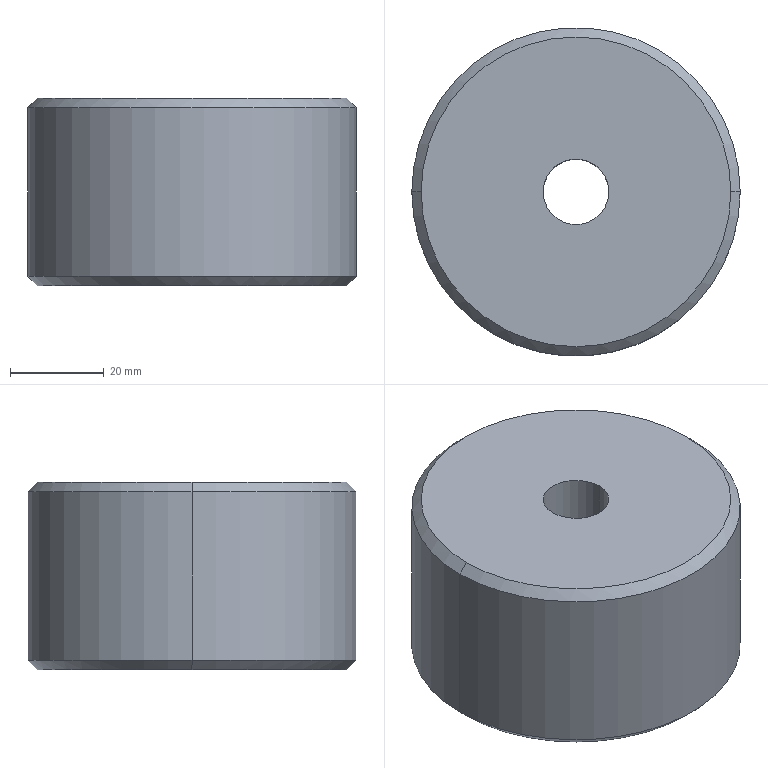Part | SolidWorks | features Chamfer 1, Extrusion 1, HoleWzd 1 | 1 solid | 10 faces | box 70 x 70 x 40 mm | volume 146918 mm3 | cylinder 4 | cone 4 | plane 2 | commonest cylinder face diameters 14 x2 70 x2
STEP:
#1=CARTESIAN_POINT('',(-7.,0.,0.));
#2=VERTEX_POINT('',#1);
#3=CARTESIAN_POINT('',(7.,0.,0.));
#4=VERTEX_POINT('',#3);
#5=CARTESIAN_POINT('',(0.,0.,0.));
#6=DIRECTION('',(0.,0.,1.));
#7=DIRECTION('',(1.,0.,0.));
#8=AXIS2_PLACEMENT_3D('',#5,#6,#7);
#9=CIRCLE('',#8,7.);
#10=EDGE_CURVE('',#2,#4,#9,.T.);
#11=ORIENTED_EDGE('',*,*,#10,.F.);
#12=CARTESIAN_POINT('',(-7.,0.,40.));
#13=VERTEX_POINT('',#12);
#14=CARTESIAN_POINT('',(-7.,0.,40.));
#15=DIRECTION('',(0.,0.,1.));
#16=VECTOR('',#15,1000.);
#17=LINE('',#14,#16);
#18=EDGE_CURVE('',#2,#13,#17,.T.);
#19=ORIENTED_EDGE('',*,*,#18,.T.);
#20=CARTESIAN_POINT('',(7.,0.,40.));
#21=VERTEX_POINT('',#20);
#22=CARTESIAN_POINT('',(0.,0.,40.));
#23=DIRECTION('',(0.,0.,1.));
#24=DIRECTION('',(1.,0.,0.));
#25=AXIS2_PLACEMENT_3D('',#22,#23,#24);
#26=CIRCLE('',#25,7.);
#27=EDGE_CURVE('',#13,#21,#26,.T.);
#28=ORIENTED_EDGE('',*,*,#27,.T.);
#29=CARTESIAN_POINT('',(7.,0.,40.));
#30=DIRECTION('',(0.,0.,1.));
#31=VECTOR('',#30,1000.);
#32=LINE('',#29,#31);
#33=EDGE_CURVE('',#4,#21,#32,.T.);
#34=ORIENTED_EDGE('',*,*,#33,.F.);
#35=EDGE_LOOP('',(#11,#19,#28,#34));
#36=FACE_OUTER_BOUND('',#35,.T.);
#37=CARTESIAN_POINT('',(0.,0.,40.));
#38=DIRECTION('',(0.,0.,1.));
#39=DIRECTION('',(1.,0.,0.));
#40=AXIS2_PLACEMENT_3D('',#37,#38,#39);
#41=CYLINDRICAL_SURFACE('',#40,7.);
#42=ADVANCED_FACE('',(#36),#41,.F.);
#43=CARTESIAN_POINT('',(33.,0.,40.));
#44=VERTEX_POINT('',#43);
#45=CARTESIAN_POINT('',(-33.,0.,40.));
#46=VERTEX_POINT('',#45);
#47=CARTESIAN_POINT('',(0.,0.,40.));
#48=DIRECTION('',(0.,0.,1.));
#49=DIRECTION('',(1.,0.,0.));
#50=AXIS2_PLACEMENT_3D('',#47,#48,#49);
#51=CIRCLE('',#50,33.);
#52=EDGE_CURVE('',#44,#46,#51,.T.);
#53=ORIENTED_EDGE('',*,*,#52,.F.);
#54=CARTESIAN_POINT('',(35.,0.,38.));
#55=VERTEX_POINT('',#54);
#56=CARTESIAN_POINT('',(33.,0.,40.));
#57=DIRECTION('',(0.7071,0.,-0.7071));
#58=VECTOR('',#57,1000.);
#59=LINE('',#56,#58);
#60=EDGE_CURVE('',#44,#55,#59,.T.);
#61=ORIENTED_EDGE('',*,*,#60,.T.);
#62=CARTESIAN_POINT('',(-35.,0.,38.));
#63=VERTEX_POINT('',#62);
#64=CARTESIAN_POINT('',(0.,0.,38.));
#65=DIRECTION('',(0.,0.,-1.));
#66=DIRECTION('',(1.,0.,0.));
#67=AXIS2_PLACEMENT_3D('',#64,#65,#66);
#68=CIRCLE('',#67,35.);
#69=EDGE_CURVE('',#63,#55,#68,.T.);
#70=ORIENTED_EDGE('',*,*,#69,.F.);
#71=CARTESIAN_POINT('',(-33.,0.,40.));
#72=DIRECTION('',(-0.7071,0.,-0.7071));
#73=VECTOR('',#72,1000.);
#74=LINE('',#71,#73);
#75=EDGE_CURVE('',#46,#63,#74,.T.);
#76=ORIENTED_EDGE('',*,*,#75,.F.);
#77=EDGE_LOOP('',(#53,#61,#70,#76));
#78=FACE_OUTER_BOUND('',#77,.T.);
#79=CARTESIAN_POINT('',(0.,0.,40.));
#80=DIRECTION('',(0.,0.,-1.));
#81=DIRECTION('',(-1.,0.,0.));
#82=AXIS2_PLACEMENT_3D('',#79,#80,#81);
#83=CONICAL_SURFACE('',#82,33.,0.7854);
#84=ADVANCED_FACE('',(#78),#83,.T.);
#85=CARTESIAN_POINT('',(-33.,0.,0.));
#86=VERTEX_POINT('',#85);
#87=CARTESIAN_POINT('',(33.,0.,0.));
#88=VERTEX_POINT('',#87);
#89=CARTESIAN_POINT('',(0.,0.,0.));
#90=DIRECTION('',(0.,0.,-1.));
#91=DIRECTION('',(1.,0.,0.));
#92=AXIS2_PLACEMENT_3D('',#89,#90,#91);
#93=CIRCLE('',#92,33.);
#94=EDGE_CURVE('',#86,#88,#93,.T.);
#95=ORIENTED_EDGE('',*,*,#94,.F.);
#96=CARTESIAN_POINT('',(-35.,0.,2.));
#97=VERTEX_POINT('',#96);
#98=CARTESIAN_POINT('',(-35.,0.,2.));
#99=DIRECTION('',(-0.7071,0.,0.7071));
#100=VECTOR('',#99,1000.);
#101=LINE('',#98,#100);
#102=EDGE_CURVE('',#86,#97,#101,.T.);
#103=ORIENTED_EDGE('',*,*,#102,.T.);
#104=CARTESIAN_POINT('',(35.,0.,2.));
#105=VERTEX_POINT('',#104);
#106=CARTESIAN_POINT('',(0.,0.,2.));
#107=DIRECTION('',(0.,0.,1.));
#108=DIRECTION('',(1.,0.,0.));
#109=AXIS2_PLACEMENT_3D('',#106,#107,#108);
#110=CIRCLE('',#109,35.);
#111=EDGE_CURVE('',#105,#97,#110,.T.);
#112=ORIENTED_EDGE('',*,*,#111,.F.);
#113=CARTESIAN_POINT('',(35.,0.,2.));
#114=DIRECTION('',(0.7071,0.,0.7071));
#115=VECTOR('',#114,1000.);
#116=LINE('',#113,#115);
#117=EDGE_CURVE('',#88,#105,#116,.T.);
#118=ORIENTED_EDGE('',*,*,#117,.F.);
#119=EDGE_LOOP('',(#95,#103,#112,#118));
#120=FACE_OUTER_BOUND('',#119,.T.);
#121=CARTESIAN_POINT('',(0.,0.,2.));
#122=DIRECTION('',(0.,0.,1.));
#123=DIRECTION('',(1.,0.,0.));
#124=AXIS2_PLACEMENT_3D('',#121,#122,#123);
#125=CONICAL_SURFACE('',#124,35.,0.7854);
#126=ADVANCED_FACE('',(#120),#125,.T.);
#127=ORIENTED_EDGE('',*,*,#69,.T.);
#128=CARTESIAN_POINT('',(35.,0.,40.));
#129=DIRECTION('',(0.,0.,-1.));
#130=VECTOR('',#129,1000.);
#131=LINE('',#128,#130);
#132=EDGE_CURVE('',#55,#105,#131,.T.);
#133=ORIENTED_EDGE('',*,*,#132,.T.);
#134=ORIENTED_EDGE('',*,*,#111,.T.);
#135=CARTESIAN_POINT('',(-35.,0.,40.));
#136=DIRECTION('',(0.,0.,-1.));
#137=VECTOR('',#136,1000.);
#138=LINE('',#135,#137);
#139=EDGE_CURVE('',#63,#97,#138,.T.);
#140=ORIENTED_EDGE('',*,*,#139,.F.);
#141=EDGE_LOOP('',(#127,#133,#134,#140));
#142=FACE_OUTER_BOUND('',#141,.T.);
#143=CARTESIAN_POINT('',(0.,0.,40.));
#144=DIRECTION('',(0.,0.,-1.));
#145=DIRECTION('',(-1.,0.,0.));
#146=AXIS2_PLACEMENT_3D('',#143,#144,#145);
#147=CYLINDRICAL_SURFACE('',#146,35.);
#148=ADVANCED_FACE('',(#142),#147,.T.);
#149=ORIENTED_EDGE('',*,*,#132,.F.);
#150=CARTESIAN_POINT('',(0.,0.,38.));
#151=DIRECTION('',(0.,0.,-1.));
#152=DIRECTION('',(1.,0.,0.));
#153=AXIS2_PLACEMENT_3D('',#150,#151,#152);
#154=CIRCLE('',#153,35.);
#155=EDGE_CURVE('',#55,#63,#154,.T.);
#156=ORIENTED_EDGE('',*,*,#155,.T.);
#157=ORIENTED_EDGE('',*,*,#139,.T.);
#158=CARTESIAN_POINT('',(0.,0.,2.));
#159=DIRECTION('',(0.,0.,1.));
#160=DIRECTION('',(1.,0.,0.));
#161=AXIS2_PLACEMENT_3D('',#158,#159,#160);
#162=CIRCLE('',#161,35.);
#163=EDGE_CURVE('',#97,#105,#162,.T.);
#164=ORIENTED_EDGE('',*,*,#163,.T.);
#165=EDGE_LOOP('',(#149,#156,#157,#164));
#166=FACE_OUTER_BOUND('',#165,.T.);
#167=CARTESIAN_POINT('',(0.,0.,40.));
#168=DIRECTION('',(0.,0.,-1.));
#169=DIRECTION('',(-1.,0.,0.));
#170=AXIS2_PLACEMENT_3D('',#167,#168,#169);
#171=CYLINDRICAL_SURFACE('',#170,35.);
#172=ADVANCED_FACE('',(#166),#171,.T.);
#173=CARTESIAN_POINT('',(0.,0.,40.));
#174=DIRECTION('',(0.,0.,1.));
#175=DIRECTION('',(1.,0.,0.));
#176=AXIS2_PLACEMENT_3D('',#173,#174,#175);
#177=CIRCLE('',#176,7.);
#178=EDGE_CURVE('',#21,#13,#177,.T.);
#179=ORIENTED_EDGE('',*,*,#178,.F.);
#180=ORIENTED_EDGE('',*,*,#27,.F.);
#181=EDGE_LOOP('',(#179,#180));
#182=FACE_BOUND('',#181,.T.);
#183=CARTESIAN_POINT('',(0.,0.,40.));
#184=DIRECTION('',(0.,0.,1.));
#185=DIRECTION('',(1.,0.,0.));
#186=AXIS2_PLACEMENT_3D('',#183,#184,#185);
#187=CIRCLE('',#186,33.);
#188=EDGE_CURVE('',#46,#44,#187,.T.);
#189=ORIENTED_EDGE('',*,*,#188,.T.);
#190=ORIENTED_EDGE('',*,*,#52,.T.);
#191=EDGE_LOOP('',(#189,#190));
#192=FACE_OUTER_BOUND('',#191,.T.);
#193=CARTESIAN_POINT('',(0.,0.,40.));
#194=DIRECTION('',(0.,0.,1.));
#195=DIRECTION('',(1.,0.,0.));
#196=AXIS2_PLACEMENT_3D('',#193,#194,#195);
#197=PLANE('',#196);
#198=ADVANCED_FACE('',(#182,#192),#197,.T.);
#199=CARTESIAN_POINT('',(0.,0.,0.));
#200=DIRECTION('',(0.,0.,1.));
#201=DIRECTION('',(1.,0.,0.));
#202=AXIS2_PLACEMENT_3D('',#199,#200,#201);
#203=CIRCLE('',#202,7.);
#204=EDGE_CURVE('',#4,#2,#203,.T.);
#205=ORIENTED_EDGE('',*,*,#204,.T.);
#206=ORIENTED_EDGE('',*,*,#10,.T.);
#207=EDGE_LOOP('',(#205,#206));
#208=FACE_BOUND('',#207,.T.);
#209=CARTESIAN_POINT('',(0.,0.,0.));
#210=DIRECTION('',(0.,0.,-1.));
#211=DIRECTION('',(1.,0.,0.));
#212=AXIS2_PLACEMENT_3D('',#209,#210,#211);
#213=CIRCLE('',#212,33.);
#214=EDGE_CURVE('',#88,#86,#213,.T.);
#215=ORIENTED_EDGE('',*,*,#214,.T.);
#216=ORIENTED_EDGE('',*,*,#94,.T.);
#217=EDGE_LOOP('',(#215,#216));
#218=FACE_OUTER_BOUND('',#217,.T.);
#219=CARTESIAN_POINT('',(0.,0.,0.));
#220=DIRECTION('',(0.,0.,1.));
#221=DIRECTION('',(1.,0.,0.));
#222=AXIS2_PLACEMENT_3D('',#219,#220,#221);
#223=PLANE('',#222);
#224=ADVANCED_FACE('',(#208,#218),#223,.F.);
#225=ORIENTED_EDGE('',*,*,#102,.F.);
#226=ORIENTED_EDGE('',*,*,#214,.F.);
#227=ORIENTED_EDGE('',*,*,#117,.T.);
#228=ORIENTED_EDGE('',*,*,#163,.F.);
#229=EDGE_LOOP('',(#225,#226,#227,#228));
#230=FACE_OUTER_BOUND('',#229,.T.);
#231=CARTESIAN_POINT('',(0.,0.,2.));
#232=DIRECTION('',(0.,0.,1.));
#233=DIRECTION('',(1.,0.,0.));
#234=AXIS2_PLACEMENT_3D('',#231,#232,#233);
#235=CONICAL_SURFACE('',#234,35.,0.7854);
#236=ADVANCED_FACE('',(#230),#235,.T.);
#237=ORIENTED_EDGE('',*,*,#60,.F.);
#238=ORIENTED_EDGE('',*,*,#188,.F.);
#239=ORIENTED_EDGE('',*,*,#75,.T.);
#240=ORIENTED_EDGE('',*,*,#155,.F.);
#241=EDGE_LOOP('',(#237,#238,#239,#240));
#242=FACE_OUTER_BOUND('',#241,.T.);
#243=CARTESIAN_POINT('',(0.,0.,40.));
#244=DIRECTION('',(0.,0.,-1.));
#245=DIRECTION('',(-1.,0.,0.));
#246=AXIS2_PLACEMENT_3D('',#243,#244,#245);
#247=CONICAL_SURFACE('',#246,33.,0.7854);
#248=ADVANCED_FACE('',(#242),#247,.T.);
#249=ORIENTED_EDGE('',*,*,#18,.F.);
#250=ORIENTED_EDGE('',*,*,#204,.F.);
#251=ORIENTED_EDGE('',*,*,#33,.T.);
#252=ORIENTED_EDGE('',*,*,#178,.T.);
#253=EDGE_LOOP('',(#249,#250,#251,#252));
#254=FACE_OUTER_BOUND('',#253,.T.);
#255=CARTESIAN_POINT('',(0.,0.,40.));
#256=DIRECTION('',(0.,0.,1.));
#257=DIRECTION('',(1.,0.,0.));
#258=AXIS2_PLACEMENT_3D('',#255,#256,#257);
#259=CYLINDRICAL_SURFACE('',#258,7.);
#260=ADVANCED_FACE('',(#254),#259,.F.);
#261=CLOSED_SHELL('',(#42,#84,#126,#148,#172,#198,#224,#236,#248,#260));
#262=MANIFOLD_SOLID_BREP('',#261);
#263=CARTESIAN_POINT('',(0.,0.,0.));
#264=DIRECTION('',(0.,0.,1.));
#265=DIRECTION('',(1.,0.,0.));
#266=AXIS2_PLACEMENT_3D('',#263,#264,#265);
#267=(LENGTH_UNIT()NAMED_UNIT(*)SI_UNIT(.MILLI.,.METRE.));
#268=UNCERTAINTY_MEASURE_WITH_UNIT(LENGTH_MEASURE(0.00001),#267,'','');
#269=(NAMED_UNIT(*)PLANE_ANGLE_UNIT()SI_UNIT($,.RADIAN.));
#270=(NAMED_UNIT(*)SI_UNIT($,.STERADIAN.)SOLID_ANGLE_UNIT());
#271=(GEOMETRIC_REPRESENTATION_CONTEXT(3)GLOBAL_UNCERTAINTY_ASSIGNED_CONTEXT((#268))GLOBAL_UNIT_ASSIGNED_CONTEXT((#267,#269,#270))REPRESENTATION_CONTEXT('',''));
#272=ADVANCED_BREP_SHAPE_REPRESENTATION('',(#262,#266),#271);